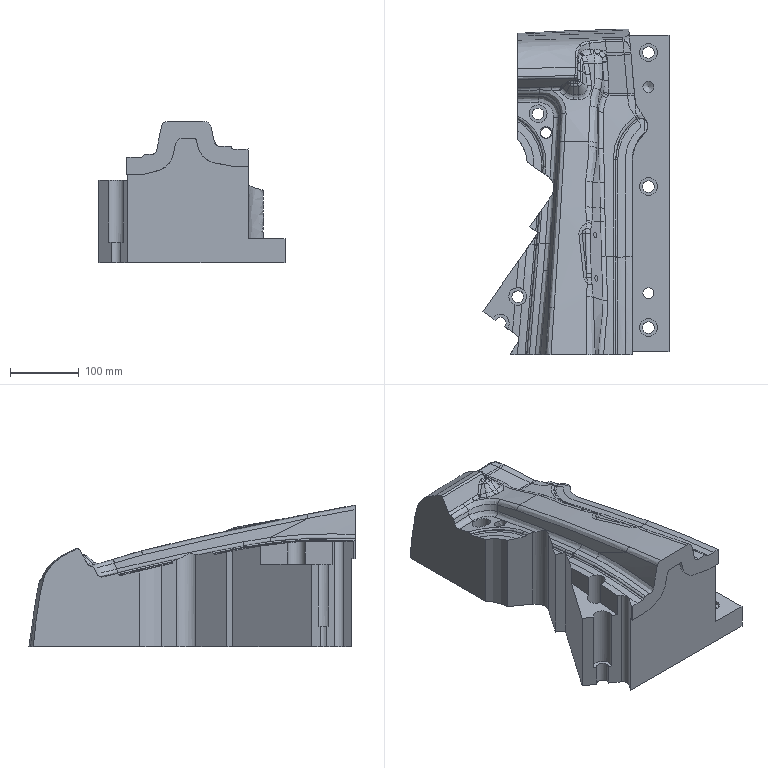Part | NX | features solid 2 | 1 solid | 272 faces | box 270.499 x 474.982 x 209.998 mm | volume 9444564 mm3 | spline 223 | plane 29 | cylinder 19 | cone 1 | commonest cylinder face diameters 17 x6 26 x6 16 x3 32 x2 20 x1 40 x1